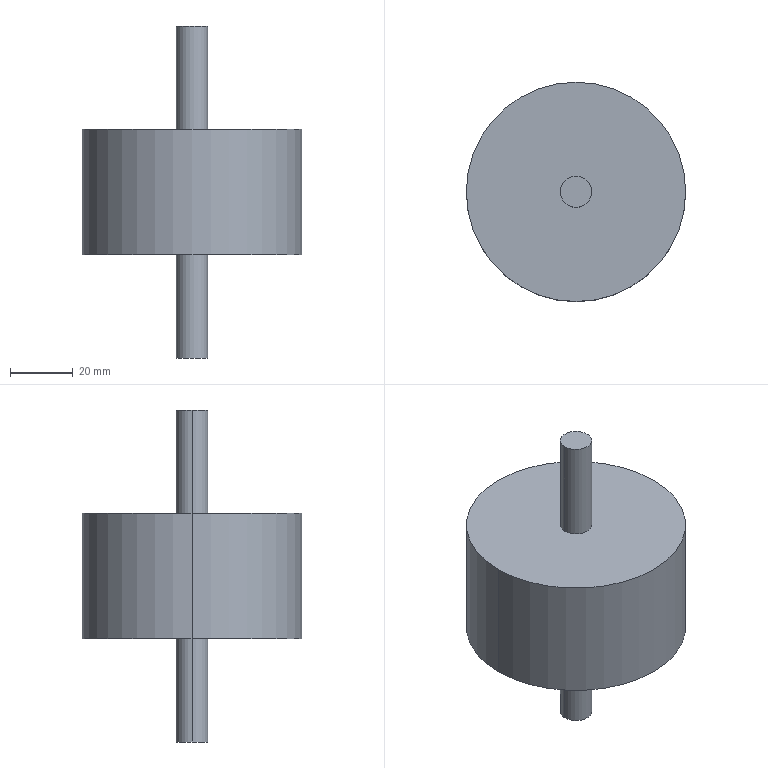Part | 1 solid | 10 faces | box 70 x 70 x 106 mm | volume 159122 mm3 | cylinder 6 | plane 4 | commonest cylinder face diameters 10 x4 70 x2
STEP:
#1=CARTESIAN_POINT('',(-5.,0.,-33.));
#2=VERTEX_POINT('',#1);
#3=CARTESIAN_POINT('',(5.,0.,-33.));
#4=VERTEX_POINT('',#3);
#5=CARTESIAN_POINT('',(0.,0.,-33.));
#6=DIRECTION('',(0.,0.,-1.));
#7=DIRECTION('',(-1.,0.,0.));
#8=AXIS2_PLACEMENT_3D('',#5,#6,#7);
#9=CIRCLE('',#8,5.);
#10=EDGE_CURVE('',#2,#4,#9,.T.);
#11=ORIENTED_EDGE('',*,*,#10,.F.);
#12=CARTESIAN_POINT('',(-5.,0.,0.));
#13=VERTEX_POINT('',#12);
#14=CARTESIAN_POINT('',(-5.,0.,-33.));
#15=DIRECTION('',(0.,0.,1.));
#16=VECTOR('',#15,1000.);
#17=LINE('',#14,#16);
#18=EDGE_CURVE('',#2,#13,#17,.T.);
#19=ORIENTED_EDGE('',*,*,#18,.T.);
#20=CARTESIAN_POINT('',(5.,0.,0.));
#21=VERTEX_POINT('',#20);
#22=CARTESIAN_POINT('',(0.,0.,0.));
#23=DIRECTION('',(0.,0.,-1.));
#24=DIRECTION('',(1.,0.,0.));
#25=AXIS2_PLACEMENT_3D('',#22,#23,#24);
#26=CIRCLE('',#25,5.);
#27=EDGE_CURVE('',#13,#21,#26,.T.);
#28=ORIENTED_EDGE('',*,*,#27,.T.);
#29=CARTESIAN_POINT('',(5.,0.,-33.));
#30=DIRECTION('',(0.,0.,1.));
#31=VECTOR('',#30,1000.);
#32=LINE('',#29,#31);
#33=EDGE_CURVE('',#4,#21,#32,.T.);
#34=ORIENTED_EDGE('',*,*,#33,.F.);
#35=EDGE_LOOP('',(#11,#19,#28,#34));
#36=FACE_OUTER_BOUND('',#35,.T.);
#37=CARTESIAN_POINT('',(0.,0.,-33.));
#38=DIRECTION('',(0.,0.,1.));
#39=DIRECTION('',(1.,0.,0.));
#40=AXIS2_PLACEMENT_3D('',#37,#38,#39);
#41=CYLINDRICAL_SURFACE('',#40,5.);
#42=ADVANCED_FACE('',(#36),#41,.T.);
#43=CARTESIAN_POINT('',(5.,0.,73.));
#44=VERTEX_POINT('',#43);
#45=CARTESIAN_POINT('',(-5.,0.,73.));
#46=VERTEX_POINT('',#45);
#47=CARTESIAN_POINT('',(0.,0.,73.));
#48=DIRECTION('',(0.,0.,1.));
#49=DIRECTION('',(1.,0.,0.));
#50=AXIS2_PLACEMENT_3D('',#47,#48,#49);
#51=CIRCLE('',#50,5.);
#52=EDGE_CURVE('',#44,#46,#51,.T.);
#53=ORIENTED_EDGE('',*,*,#52,.F.);
#54=CARTESIAN_POINT('',(5.,0.,40.));
#55=VERTEX_POINT('',#54);
#56=CARTESIAN_POINT('',(5.,0.,73.));
#57=DIRECTION('',(0.,0.,-1.));
#58=VECTOR('',#57,1000.);
#59=LINE('',#56,#58);
#60=EDGE_CURVE('',#44,#55,#59,.T.);
#61=ORIENTED_EDGE('',*,*,#60,.T.);
#62=CARTESIAN_POINT('',(-5.,0.,40.));
#63=VERTEX_POINT('',#62);
#64=CARTESIAN_POINT('',(0.,0.,40.));
#65=DIRECTION('',(0.,0.,1.));
#66=DIRECTION('',(1.,0.,0.));
#67=AXIS2_PLACEMENT_3D('',#64,#65,#66);
#68=CIRCLE('',#67,5.);
#69=EDGE_CURVE('',#55,#63,#68,.T.);
#70=ORIENTED_EDGE('',*,*,#69,.T.);
#71=CARTESIAN_POINT('',(-5.,0.,73.));
#72=DIRECTION('',(0.,0.,-1.));
#73=VECTOR('',#72,1000.);
#74=LINE('',#71,#73);
#75=EDGE_CURVE('',#46,#63,#74,.T.);
#76=ORIENTED_EDGE('',*,*,#75,.F.);
#77=EDGE_LOOP('',(#53,#61,#70,#76));
#78=FACE_OUTER_BOUND('',#77,.T.);
#79=CARTESIAN_POINT('',(0.,0.,73.));
#80=DIRECTION('',(0.,0.,-1.));
#81=DIRECTION('',(-1.,0.,0.));
#82=AXIS2_PLACEMENT_3D('',#79,#80,#81);
#83=CYLINDRICAL_SURFACE('',#82,5.);
#84=ADVANCED_FACE('',(#78),#83,.T.);
#85=CARTESIAN_POINT('',(35.,0.,40.));
#86=VERTEX_POINT('',#85);
#87=CARTESIAN_POINT('',(-35.,0.,40.));
#88=VERTEX_POINT('',#87);
#89=CARTESIAN_POINT('',(0.,0.,40.));
#90=DIRECTION('',(0.,0.,1.));
#91=DIRECTION('',(1.,0.,0.));
#92=AXIS2_PLACEMENT_3D('',#89,#90,#91);
#93=CIRCLE('',#92,35.);
#94=EDGE_CURVE('',#86,#88,#93,.T.);
#95=ORIENTED_EDGE('',*,*,#94,.F.);
#96=CARTESIAN_POINT('',(35.,0.,0.));
#97=VERTEX_POINT('',#96);
#98=CARTESIAN_POINT('',(35.,0.,40.));
#99=DIRECTION('',(0.,0.,-1.));
#100=VECTOR('',#99,1000.);
#101=LINE('',#98,#100);
#102=EDGE_CURVE('',#86,#97,#101,.T.);
#103=ORIENTED_EDGE('',*,*,#102,.T.);
#104=CARTESIAN_POINT('',(-35.,0.,0.));
#105=VERTEX_POINT('',#104);
#106=CARTESIAN_POINT('',(0.,0.,0.));
#107=DIRECTION('',(0.,0.,1.));
#108=DIRECTION('',(1.,0.,0.));
#109=AXIS2_PLACEMENT_3D('',#106,#107,#108);
#110=CIRCLE('',#109,35.);
#111=EDGE_CURVE('',#97,#105,#110,.T.);
#112=ORIENTED_EDGE('',*,*,#111,.T.);
#113=CARTESIAN_POINT('',(-35.,0.,40.));
#114=DIRECTION('',(0.,0.,-1.));
#115=VECTOR('',#114,1000.);
#116=LINE('',#113,#115);
#117=EDGE_CURVE('',#88,#105,#116,.T.);
#118=ORIENTED_EDGE('',*,*,#117,.F.);
#119=EDGE_LOOP('',(#95,#103,#112,#118));
#120=FACE_OUTER_BOUND('',#119,.T.);
#121=CARTESIAN_POINT('',(0.,0.,40.));
#122=DIRECTION('',(0.,0.,-1.));
#123=DIRECTION('',(-1.,0.,0.));
#124=AXIS2_PLACEMENT_3D('',#121,#122,#123);
#125=CYLINDRICAL_SURFACE('',#124,35.);
#126=ADVANCED_FACE('',(#120),#125,.T.);
#127=ORIENTED_EDGE('',*,*,#102,.F.);
#128=CARTESIAN_POINT('',(0.,0.,40.));
#129=DIRECTION('',(0.,0.,1.));
#130=DIRECTION('',(1.,0.,0.));
#131=AXIS2_PLACEMENT_3D('',#128,#129,#130);
#132=CIRCLE('',#131,35.);
#133=EDGE_CURVE('',#88,#86,#132,.T.);
#134=ORIENTED_EDGE('',*,*,#133,.F.);
#135=ORIENTED_EDGE('',*,*,#117,.T.);
#136=CARTESIAN_POINT('',(0.,0.,0.));
#137=DIRECTION('',(0.,0.,1.));
#138=DIRECTION('',(1.,0.,0.));
#139=AXIS2_PLACEMENT_3D('',#136,#137,#138);
#140=CIRCLE('',#139,35.);
#141=EDGE_CURVE('',#105,#97,#140,.T.);
#142=ORIENTED_EDGE('',*,*,#141,.T.);
#143=EDGE_LOOP('',(#127,#134,#135,#142));
#144=FACE_OUTER_BOUND('',#143,.T.);
#145=CARTESIAN_POINT('',(0.,0.,40.));
#146=DIRECTION('',(0.,0.,-1.));
#147=DIRECTION('',(-1.,0.,0.));
#148=AXIS2_PLACEMENT_3D('',#145,#146,#147);
#149=CYLINDRICAL_SURFACE('',#148,35.);
#150=ADVANCED_FACE('',(#144),#149,.T.);
#151=CARTESIAN_POINT('',(0.,0.,40.));
#152=DIRECTION('',(0.,0.,1.));
#153=DIRECTION('',(1.,0.,0.));
#154=AXIS2_PLACEMENT_3D('',#151,#152,#153);
#155=CIRCLE('',#154,5.);
#156=EDGE_CURVE('',#63,#55,#155,.T.);
#157=ORIENTED_EDGE('',*,*,#156,.F.);
#158=ORIENTED_EDGE('',*,*,#69,.F.);
#159=EDGE_LOOP('',(#157,#158));
#160=FACE_BOUND('',#159,.T.);
#161=ORIENTED_EDGE('',*,*,#133,.T.);
#162=ORIENTED_EDGE('',*,*,#94,.T.);
#163=EDGE_LOOP('',(#161,#162));
#164=FACE_OUTER_BOUND('',#163,.T.);
#165=CARTESIAN_POINT('',(0.,0.,40.));
#166=DIRECTION('',(0.,0.,1.));
#167=DIRECTION('',(1.,0.,0.));
#168=AXIS2_PLACEMENT_3D('',#165,#166,#167);
#169=PLANE('',#168);
#170=ADVANCED_FACE('',(#160,#164),#169,.T.);
#171=CARTESIAN_POINT('',(0.,0.,0.));
#172=DIRECTION('',(0.,0.,-1.));
#173=DIRECTION('',(1.,0.,0.));
#174=AXIS2_PLACEMENT_3D('',#171,#172,#173);
#175=CIRCLE('',#174,5.);
#176=EDGE_CURVE('',#21,#13,#175,.T.);
#177=ORIENTED_EDGE('',*,*,#176,.F.);
#178=ORIENTED_EDGE('',*,*,#27,.F.);
#179=EDGE_LOOP('',(#177,#178));
#180=FACE_BOUND('',#179,.T.);
#181=ORIENTED_EDGE('',*,*,#141,.F.);
#182=ORIENTED_EDGE('',*,*,#111,.F.);
#183=EDGE_LOOP('',(#181,#182));
#184=FACE_OUTER_BOUND('',#183,.T.);
#185=CARTESIAN_POINT('',(0.,0.,0.));
#186=DIRECTION('',(0.,0.,1.));
#187=DIRECTION('',(1.,0.,0.));
#188=AXIS2_PLACEMENT_3D('',#185,#186,#187);
#189=PLANE('',#188);
#190=ADVANCED_FACE('',(#180,#184),#189,.F.);
#191=ORIENTED_EDGE('',*,*,#60,.F.);
#192=CARTESIAN_POINT('',(0.,0.,73.));
#193=DIRECTION('',(0.,0.,1.));
#194=DIRECTION('',(1.,0.,0.));
#195=AXIS2_PLACEMENT_3D('',#192,#193,#194);
#196=CIRCLE('',#195,5.);
#197=EDGE_CURVE('',#46,#44,#196,.T.);
#198=ORIENTED_EDGE('',*,*,#197,.F.);
#199=ORIENTED_EDGE('',*,*,#75,.T.);
#200=ORIENTED_EDGE('',*,*,#156,.T.);
#201=EDGE_LOOP('',(#191,#198,#199,#200));
#202=FACE_OUTER_BOUND('',#201,.T.);
#203=CARTESIAN_POINT('',(0.,0.,73.));
#204=DIRECTION('',(0.,0.,-1.));
#205=DIRECTION('',(-1.,0.,0.));
#206=AXIS2_PLACEMENT_3D('',#203,#204,#205);
#207=CYLINDRICAL_SURFACE('',#206,5.);
#208=ADVANCED_FACE('',(#202),#207,.T.);
#209=ORIENTED_EDGE('',*,*,#197,.T.);
#210=ORIENTED_EDGE('',*,*,#52,.T.);
#211=EDGE_LOOP('',(#209,#210));
#212=FACE_OUTER_BOUND('',#211,.T.);
#213=CARTESIAN_POINT('',(0.,0.,73.));
#214=DIRECTION('',(0.,0.,1.));
#215=DIRECTION('',(1.,0.,0.));
#216=AXIS2_PLACEMENT_3D('',#213,#214,#215);
#217=PLANE('',#216);
#218=ADVANCED_FACE('',(#212),#217,.T.);
#219=ORIENTED_EDGE('',*,*,#18,.F.);
#220=CARTESIAN_POINT('',(0.,0.,-33.));
#221=DIRECTION('',(0.,0.,-1.));
#222=DIRECTION('',(-1.,0.,0.));
#223=AXIS2_PLACEMENT_3D('',#220,#221,#222);
#224=CIRCLE('',#223,5.);
#225=EDGE_CURVE('',#4,#2,#224,.T.);
#226=ORIENTED_EDGE('',*,*,#225,.F.);
#227=ORIENTED_EDGE('',*,*,#33,.T.);
#228=ORIENTED_EDGE('',*,*,#176,.T.);
#229=EDGE_LOOP('',(#219,#226,#227,#228));
#230=FACE_OUTER_BOUND('',#229,.T.);
#231=CARTESIAN_POINT('',(0.,0.,-33.));
#232=DIRECTION('',(0.,0.,1.));
#233=DIRECTION('',(1.,0.,0.));
#234=AXIS2_PLACEMENT_3D('',#231,#232,#233);
#235=CYLINDRICAL_SURFACE('',#234,5.);
#236=ADVANCED_FACE('',(#230),#235,.T.);
#237=ORIENTED_EDGE('',*,*,#225,.T.);
#238=ORIENTED_EDGE('',*,*,#10,.T.);
#239=EDGE_LOOP('',(#237,#238));
#240=FACE_OUTER_BOUND('',#239,.T.);
#241=CARTESIAN_POINT('',(0.,0.,-33.));
#242=DIRECTION('',(0.,0.,-1.));
#243=DIRECTION('',(-1.,0.,0.));
#244=AXIS2_PLACEMENT_3D('',#241,#242,#243);
#245=PLANE('',#244);
#246=ADVANCED_FACE('',(#240),#245,.T.);
#247=CLOSED_SHELL('',(#42,#84,#126,#150,#170,#190,#208,#218,#236,#246));
#248=MANIFOLD_SOLID_BREP('',#247);
#249=CARTESIAN_POINT('',(0.,0.,0.));
#250=DIRECTION('',(0.,0.,1.));
#251=DIRECTION('',(1.,0.,0.));
#252=AXIS2_PLACEMENT_3D('',#249,#250,#251);
#253=(LENGTH_UNIT()NAMED_UNIT(*)SI_UNIT(.MILLI.,.METRE.));
#254=UNCERTAINTY_MEASURE_WITH_UNIT(LENGTH_MEASURE(0.00001),#253,'','');
#255=(NAMED_UNIT(*)PLANE_ANGLE_UNIT()SI_UNIT($,.RADIAN.));
#256=(NAMED_UNIT(*)SI_UNIT($,.STERADIAN.)SOLID_ANGLE_UNIT());
#257=(GEOMETRIC_REPRESENTATION_CONTEXT(3)GLOBAL_UNCERTAINTY_ASSIGNED_CONTEXT((#254))GLOBAL_UNIT_ASSIGNED_CONTEXT((#253,#255,#256))REPRESENTATION_CONTEXT('',''));
#258=ADVANCED_BREP_SHAPE_REPRESENTATION('',(#248,#252),#257);